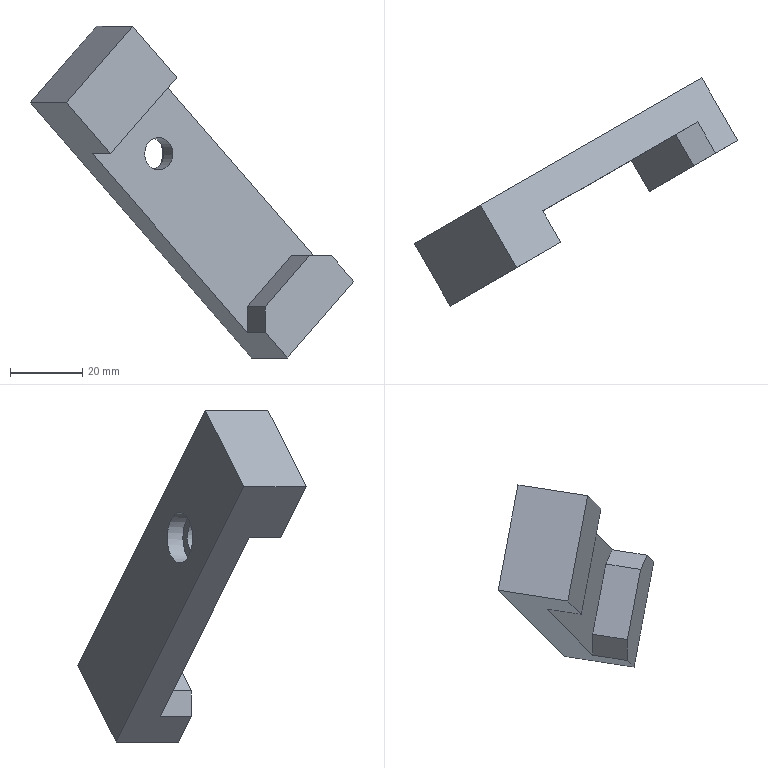Part | NX | features solid 2 | 1 solid | 15 faces | box 89.608 x 63.282 x 91.924 mm | volume 39162 mm3 | plane 13 | cylinder 2 | commonest cylinder face diameters 9 x1 14 x1
STEP:
#1=CARTESIAN_POINT('',(-1037.635,96.451,136.492));
#2=VERTEX_POINT('',#1);
#3=CARTESIAN_POINT('',(-1027.635,79.131,136.492));
#4=VERTEX_POINT('',#3);
#5=CARTESIAN_POINT('',(-1030.135,83.461,136.492));
#6=DIRECTION('',(0.5,-0.866,0.));
#7=VECTOR('',#6,1000.);
#8=LINE('',#5,#7);
#9=EDGE_CURVE('',#2,#4,#8,.T.);
#10=ORIENTED_EDGE('',*,*,#9,.T.);
#11=CARTESIAN_POINT('',(-1015.387,86.202,122.35));
#12=VERTEX_POINT('',#11);
#13=CARTESIAN_POINT('',(-1015.387,86.202,122.35));
#14=DIRECTION('',(-0.6124,-0.3536,0.7071));
#15=VECTOR('',#14,1000.);
#16=LINE('',#13,#15);
#17=EDGE_CURVE('',#4,#12,#16,.F.);
#18=ORIENTED_EDGE('',*,*,#17,.T.);
#19=CARTESIAN_POINT('',(-1020.387,94.862,122.35));
#20=VERTEX_POINT('',#19);
#21=CARTESIAN_POINT('',(-1017.887,90.532,122.35));
#22=DIRECTION('',(0.5,-0.866,0.));
#23=VECTOR('',#22,1000.);
#24=LINE('',#21,#23);
#25=EDGE_CURVE('',#20,#12,#24,.T.);
#26=ORIENTED_EDGE('',*,*,#25,.F.);
#27=CARTESIAN_POINT('',(-977.521,119.611,72.852));
#28=VERTEX_POINT('',#27);
#29=CARTESIAN_POINT('',(-1020.387,94.862,122.35));
#30=DIRECTION('',(-0.6124,-0.3536,0.7071));
#31=VECTOR('',#30,1000.);
#32=LINE('',#29,#31);
#33=EDGE_CURVE('',#20,#28,#32,.F.);
#34=ORIENTED_EDGE('',*,*,#33,.T.);
#35=CARTESIAN_POINT('',(-972.521,110.95,72.852));
#36=VERTEX_POINT('',#35);
#37=CARTESIAN_POINT('',(-975.021,115.28,72.852));
#38=DIRECTION('',(-0.5,0.866,0.));
#39=VECTOR('',#38,1000.);
#40=LINE('',#37,#39);
#41=EDGE_CURVE('',#36,#28,#40,.T.);
#42=ORIENTED_EDGE('',*,*,#41,.F.);
#43=CARTESIAN_POINT('',(-966.398,114.486,65.781));
#44=VERTEX_POINT('',#43);
#45=CARTESIAN_POINT('',(-1015.387,86.202,122.35));
#46=DIRECTION('',(0.6124,0.3536,-0.7071));
#47=VECTOR('',#46,1000.);
#48=LINE('',#45,#47);
#49=EDGE_CURVE('',#44,#36,#48,.F.);
#50=ORIENTED_EDGE('',*,*,#49,.F.);
#51=CARTESIAN_POINT('',(-976.398,131.806,65.781));
#52=VERTEX_POINT('',#51);
#53=CARTESIAN_POINT('',(-968.898,118.816,65.781));
#54=DIRECTION('',(0.5,-0.866,0.));
#55=VECTOR('',#54,1000.);
#56=LINE('',#53,#55);
#57=EDGE_CURVE('',#52,#44,#56,.T.);
#58=ORIENTED_EDGE('',*,*,#57,.F.);
#59=CARTESIAN_POINT('',(-1025.387,103.522,122.35));
#60=DIRECTION('',(-0.6124,-0.3536,0.7071));
#61=VECTOR('',#60,1000.);
#62=LINE('',#59,#61);
#63=EDGE_CURVE('',#52,#2,#62,.T.);
#64=ORIENTED_EDGE('',*,*,#63,.T.);
#65=EDGE_LOOP('',(#10,#18,#26,#34,#42,#50,#58,#64));
#66=FACE_BOUND('',#65,.T.);
#67=CARTESIAN_POINT('',(-1017.887,90.532,122.35));
#68=DIRECTION('',(0.6124,0.3536,0.7071));
#69=DIRECTION('',(0.5,-0.866,0.));
#70=AXIS2_PLACEMENT_3D('',#67,#68,#69);
#71=PLANE('',#70);
#72=ADVANCED_FACE('',(#66),#71,.T.);
#73=CARTESIAN_POINT('',(-1038.759,84.255,101.136));
#74=VERTEX_POINT('',#73);
#75=CARTESIAN_POINT('',(-1033.759,75.595,101.136));
#76=VERTEX_POINT('',#75);
#77=CARTESIAN_POINT('',(-1036.259,79.925,101.136));
#78=DIRECTION('',(-0.5,0.866,0.));
#79=VECTOR('',#78,1000.);
#80=LINE('',#77,#79);
#81=EDGE_CURVE('',#74,#76,#80,.F.);
#82=ORIENTED_EDGE('',*,*,#81,.T.);
#83=CARTESIAN_POINT('',(-1046.006,68.524,115.279));
#84=VERTEX_POINT('',#83);
#85=CARTESIAN_POINT('',(-1033.759,75.595,101.136));
#86=DIRECTION('',(-0.6124,-0.3536,0.7071));
#87=VECTOR('',#86,1000.);
#88=LINE('',#85,#87);
#89=EDGE_CURVE('',#76,#84,#88,.T.);
#90=ORIENTED_EDGE('',*,*,#89,.T.);
#91=CARTESIAN_POINT('',(-1056.006,85.844,115.279));
#92=VERTEX_POINT('',#91);
#93=CARTESIAN_POINT('',(-1048.506,72.854,115.279));
#94=DIRECTION('',(-0.5,0.866,0.));
#95=VECTOR('',#94,1000.);
#96=LINE('',#93,#95);
#97=EDGE_CURVE('',#92,#84,#96,.F.);
#98=ORIENTED_EDGE('',*,*,#97,.F.);
#99=CARTESIAN_POINT('',(-994.769,121.2,44.568));
#100=VERTEX_POINT('',#99);
#101=CARTESIAN_POINT('',(-1043.759,92.916,101.136));
#102=DIRECTION('',(0.6124,0.3536,-0.7071));
#103=VECTOR('',#102,1000.);
#104=LINE('',#101,#103);
#105=EDGE_CURVE('',#100,#92,#104,.F.);
#106=ORIENTED_EDGE('',*,*,#105,.F.);
#107=CARTESIAN_POINT('',(-984.769,103.879,44.568));
#108=VERTEX_POINT('',#107);
#109=CARTESIAN_POINT('',(-987.269,108.209,44.568));
#110=DIRECTION('',(-0.5,0.866,0.));
#111=VECTOR('',#110,1000.);
#112=LINE('',#109,#111);
#113=EDGE_CURVE('',#100,#108,#112,.F.);
#114=ORIENTED_EDGE('',*,*,#113,.T.);
#115=CARTESIAN_POINT('',(-990.893,100.344,51.639));
#116=VERTEX_POINT('',#115);
#117=CARTESIAN_POINT('',(-1033.759,75.595,101.136));
#118=DIRECTION('',(-0.6124,-0.3536,0.7071));
#119=VECTOR('',#118,1000.);
#120=LINE('',#117,#119);
#121=EDGE_CURVE('',#108,#116,#120,.T.);
#122=ORIENTED_EDGE('',*,*,#121,.T.);
#123=CARTESIAN_POINT('',(-995.893,109.004,51.639));
#124=VERTEX_POINT('',#123);
#125=CARTESIAN_POINT('',(-993.393,104.674,51.639));
#126=DIRECTION('',(-0.5,0.866,0.));
#127=VECTOR('',#126,1000.);
#128=LINE('',#125,#127);
#129=EDGE_CURVE('',#124,#116,#128,.F.);
#130=ORIENTED_EDGE('',*,*,#129,.F.);
#131=CARTESIAN_POINT('',(-1038.759,84.255,101.136));
#132=DIRECTION('',(0.6124,0.3536,-0.7071));
#133=VECTOR('',#132,1000.);
#134=LINE('',#131,#133);
#135=EDGE_CURVE('',#74,#124,#134,.T.);
#136=ORIENTED_EDGE('',*,*,#135,.F.);
#137=EDGE_LOOP('',(#82,#90,#98,#106,#114,#122,#130,#136));
#138=FACE_BOUND('',#137,.T.);
#139=CARTESIAN_POINT('',(-1036.259,79.925,101.136));
#140=DIRECTION('',(0.6124,0.3536,0.7071));
#141=DIRECTION('',(0.5,-0.866,0.));
#142=AXIS2_PLACEMENT_3D('',#139,#140,#141);
#143=PLANE('',#142);
#144=ADVANCED_FACE('',(#138),#143,.F.);
#145=ORIENTED_EDGE('',*,*,#97,.T.);
#146=CARTESIAN_POINT('',(-1052.13,64.988,108.208));
#147=DIRECTION('',(-0.6124,-0.3536,-0.7071));
#148=VECTOR('',#147,1000.);
#149=LINE('',#146,#148);
#150=EDGE_CURVE('',#84,#4,#149,.F.);
#151=ORIENTED_EDGE('',*,*,#150,.T.);
#152=ORIENTED_EDGE('',*,*,#9,.F.);
#153=CARTESIAN_POINT('',(-1062.13,82.309,108.208));
#154=DIRECTION('',(0.6124,0.3536,0.7071));
#155=VECTOR('',#154,1000.);
#156=LINE('',#153,#155);
#157=EDGE_CURVE('',#92,#2,#156,.T.);
#158=ORIENTED_EDGE('',*,*,#157,.F.);
#159=EDGE_LOOP('',(#145,#151,#152,#158));
#160=FACE_BOUND('',#159,.T.);
#161=CARTESIAN_POINT('',(-1054.63,69.319,108.208));
#162=DIRECTION('',(-0.6124,-0.3536,0.7071));
#163=DIRECTION('',(0.6124,0.3536,0.7071));
#164=AXIS2_PLACEMENT_3D('',#161,#162,#163);
#165=PLANE('',#164);
#166=ADVANCED_FACE('',(#160),#165,.T.);
#167=CARTESIAN_POINT('',(-1039.882,72.059,94.065));
#168=DIRECTION('',(-0.6124,-0.3536,-0.7071));
#169=VECTOR('',#168,1000.);
#170=LINE('',#167,#169);
#171=EDGE_CURVE('',#76,#12,#170,.F.);
#172=ORIENTED_EDGE('',*,*,#171,.F.);
#173=ORIENTED_EDGE('',*,*,#81,.F.);
#174=CARTESIAN_POINT('',(-1044.882,80.72,94.065));
#175=DIRECTION('',(-0.6124,-0.3536,-0.7071));
#176=VECTOR('',#175,1000.);
#177=LINE('',#174,#176);
#178=EDGE_CURVE('',#74,#20,#177,.F.);
#179=ORIENTED_EDGE('',*,*,#178,.T.);
#180=ORIENTED_EDGE('',*,*,#25,.T.);
#181=EDGE_LOOP('',(#172,#173,#179,#180));
#182=FACE_BOUND('',#181,.T.);
#183=CARTESIAN_POINT('',(-1042.382,76.39,94.065));
#184=DIRECTION('',(-0.6124,-0.3536,0.7071));
#185=DIRECTION('',(0.6124,0.3536,0.7071));
#186=AXIS2_PLACEMENT_3D('',#183,#184,#185);
#187=PLANE('',#186);
#188=ADVANCED_FACE('',(#182),#187,.F.);
#189=ORIENTED_EDGE('',*,*,#121,.F.);
#190=CARTESIAN_POINT('',(-990.893,100.344,37.497));
#191=DIRECTION('',(-0.6124,-0.3536,-0.7071));
#192=VECTOR('',#191,1000.);
#193=LINE('',#190,#192);
#194=EDGE_CURVE('',#108,#44,#193,.F.);
#195=ORIENTED_EDGE('',*,*,#194,.T.);
#196=ORIENTED_EDGE('',*,*,#49,.T.);
#197=CARTESIAN_POINT('',(-978.645,107.415,72.852));
#198=VERTEX_POINT('',#197);
#199=CARTESIAN_POINT('',(-978.645,107.415,72.852));
#200=DIRECTION('',(0.866,0.5,0.));
#201=VECTOR('',#200,1000.);
#202=LINE('',#199,#201);
#203=EDGE_CURVE('',#198,#36,#202,.T.);
#204=ORIENTED_EDGE('',*,*,#203,.F.);
#205=CARTESIAN_POINT('',(-990.893,100.344,58.71));
#206=VERTEX_POINT('',#205);
#207=CARTESIAN_POINT('',(-1000.078,95.04,48.103));
#208=DIRECTION('',(-0.6124,-0.3536,-0.7071));
#209=VECTOR('',#208,1000.);
#210=LINE('',#207,#209);
#211=EDGE_CURVE('',#206,#198,#210,.F.);
#212=ORIENTED_EDGE('',*,*,#211,.F.);
#213=CARTESIAN_POINT('',(-990.893,100.344,51.639));
#214=DIRECTION('',(0.,0.,-1.));
#215=VECTOR('',#214,1000.);
#216=LINE('',#213,#215);
#217=EDGE_CURVE('',#116,#206,#216,.F.);
#218=ORIENTED_EDGE('',*,*,#217,.F.);
#219=EDGE_LOOP('',(#189,#195,#196,#204,#212,#218));
#220=FACE_BOUND('',#219,.T.);
#221=CARTESIAN_POINT('',(-1039.882,72.059,94.065));
#222=DIRECTION('',(-0.5,0.866,0.));
#223=DIRECTION('',(0.6124,0.3536,0.7071));
#224=AXIS2_PLACEMENT_3D('',#221,#222,#223);
#225=PLANE('',#224);
#226=ADVANCED_FACE('',(#220),#225,.F.);
#227=CARTESIAN_POINT('',(-1025.916,103.217,108.11));
#228=VERTEX_POINT('',#227);
#229=CARTESIAN_POINT('',(-1025.387,103.522,101.136));
#230=DIRECTION('',(-0.5,0.866,0.));
#231=DIRECTION('',(-0.07548,-0.04358,0.9962));
#232=AXIS2_PLACEMENT_3D('',#229,#230,#231);
#233=CIRCLE('',#232,7.);
#234=EDGE_CURVE('',#228,#228,#233,.T.);
#235=ORIENTED_EDGE('',*,*,#234,.F.);
#236=EDGE_LOOP('',(#235));
#237=FACE_BOUND('',#236,.T.);
#238=ORIENTED_EDGE('',*,*,#105,.T.);
#239=ORIENTED_EDGE('',*,*,#157,.T.);
#240=ORIENTED_EDGE('',*,*,#63,.F.);
#241=CARTESIAN_POINT('',(-1000.893,117.664,37.497));
#242=DIRECTION('',(0.6124,0.3536,0.7071));
#243=VECTOR('',#242,1000.);
#244=LINE('',#241,#243);
#245=EDGE_CURVE('',#100,#52,#244,.T.);
#246=ORIENTED_EDGE('',*,*,#245,.F.);
#247=EDGE_LOOP('',(#238,#239,#240,#246));
#248=FACE_BOUND('',#247,.T.);
#249=CARTESIAN_POINT('',(-1049.882,89.38,94.065));
#250=DIRECTION('',(-0.5,0.866,0.));
#251=DIRECTION('',(0.6124,0.3536,0.7071));
#252=AXIS2_PLACEMENT_3D('',#249,#250,#251);
#253=PLANE('',#252);
#254=ADVANCED_FACE('',(#237,#248),#253,.T.);
#255=ORIENTED_EDGE('',*,*,#194,.F.);
#256=ORIENTED_EDGE('',*,*,#113,.F.);
#257=ORIENTED_EDGE('',*,*,#245,.T.);
#258=ORIENTED_EDGE('',*,*,#57,.T.);
#259=EDGE_LOOP('',(#255,#256,#257,#258));
#260=FACE_BOUND('',#259,.T.);
#261=CARTESIAN_POINT('',(-993.393,104.674,37.497));
#262=DIRECTION('',(-0.6124,-0.3536,0.7071));
#263=DIRECTION('',(0.6124,0.3536,0.7071));
#264=AXIS2_PLACEMENT_3D('',#261,#262,#263);
#265=PLANE('',#264);
#266=ADVANCED_FACE('',(#260),#265,.F.);
#267=CARTESIAN_POINT('',(-983.645,116.075,72.852));
#268=VERTEX_POINT('',#267);
#269=CARTESIAN_POINT('',(-1044.882,80.72,72.852));
#270=DIRECTION('',(-0.866,-0.5,0.));
#271=VECTOR('',#270,1000.);
#272=LINE('',#269,#271);
#273=EDGE_CURVE('',#28,#268,#272,.T.);
#274=ORIENTED_EDGE('',*,*,#273,.F.);
#275=ORIENTED_EDGE('',*,*,#33,.F.);
#276=ORIENTED_EDGE('',*,*,#178,.F.);
#277=ORIENTED_EDGE('',*,*,#135,.T.);
#278=CARTESIAN_POINT('',(-995.893,109.004,58.71));
#279=VERTEX_POINT('',#278);
#280=CARTESIAN_POINT('',(-995.893,109.004,94.065));
#281=DIRECTION('',(0.,0.,1.));
#282=VECTOR('',#281,1000.);
#283=LINE('',#280,#282);
#284=EDGE_CURVE('',#279,#124,#283,.F.);
#285=ORIENTED_EDGE('',*,*,#284,.F.);
#286=CARTESIAN_POINT('',(-1005.078,103.701,48.103));
#287=DIRECTION('',(-0.6124,-0.3536,-0.7071));
#288=VECTOR('',#287,1000.);
#289=LINE('',#286,#288);
#290=EDGE_CURVE('',#279,#268,#289,.F.);
#291=ORIENTED_EDGE('',*,*,#290,.T.);
#292=EDGE_LOOP('',(#274,#275,#276,#277,#285,#291));
#293=FACE_BOUND('',#292,.T.);
#294=CARTESIAN_POINT('',(-1024.27,92.62,101.529));
#295=VERTEX_POINT('',#294);
#296=CARTESIAN_POINT('',(-1020.387,94.862,101.136));
#297=DIRECTION('',(-0.5,0.866,0.));
#298=DIRECTION('',(-0.8627,-0.4981,0.08716));
#299=AXIS2_PLACEMENT_3D('',#296,#297,#298);
#300=CIRCLE('',#299,4.5);
#301=EDGE_CURVE('',#295,#295,#300,.T.);
#302=ORIENTED_EDGE('',*,*,#301,.T.);
#303=EDGE_LOOP('',(#302));
#304=FACE_BOUND('',#303,.T.);
#305=CARTESIAN_POINT('',(-1044.882,80.72,94.065));
#306=DIRECTION('',(-0.5,0.866,0.));
#307=DIRECTION('',(0.6124,0.3536,0.7071));
#308=AXIS2_PLACEMENT_3D('',#305,#306,#307);
#309=PLANE('',#308);
#310=ADVANCED_FACE('',(#293,#304),#309,.F.);
#311=ORIENTED_EDGE('',*,*,#211,.T.);
#312=CARTESIAN_POINT('',(-981.145,111.745,72.852));
#313=DIRECTION('',(0.5,-0.866,0.));
#314=VECTOR('',#313,1000.);
#315=LINE('',#312,#314);
#316=EDGE_CURVE('',#268,#198,#315,.T.);
#317=ORIENTED_EDGE('',*,*,#316,.F.);
#318=ORIENTED_EDGE('',*,*,#290,.F.);
#319=CARTESIAN_POINT('',(-993.393,104.674,58.71));
#320=DIRECTION('',(-0.5,0.866,0.));
#321=VECTOR('',#320,1000.);
#322=LINE('',#319,#321);
#323=EDGE_CURVE('',#206,#279,#322,.T.);
#324=ORIENTED_EDGE('',*,*,#323,.F.);
#325=EDGE_LOOP('',(#311,#317,#318,#324));
#326=FACE_BOUND('',#325,.T.);
#327=CARTESIAN_POINT('',(-1002.578,99.371,48.103));
#328=DIRECTION('',(-0.6124,-0.3536,0.7071));
#329=DIRECTION('',(0.6124,0.3536,0.7071));
#330=AXIS2_PLACEMENT_3D('',#327,#328,#329);
#331=PLANE('',#330);
#332=ADVANCED_FACE('',(#326),#331,.T.);
#333=ORIENTED_EDGE('',*,*,#284,.T.);
#334=ORIENTED_EDGE('',*,*,#129,.T.);
#335=ORIENTED_EDGE('',*,*,#217,.T.);
#336=ORIENTED_EDGE('',*,*,#323,.T.);
#337=EDGE_LOOP('',(#333,#334,#335,#336));
#338=FACE_BOUND('',#337,.T.);
#339=CARTESIAN_POINT('',(-993.393,104.674,51.639));
#340=DIRECTION('',(-0.866,-0.5,0.));
#341=DIRECTION('',(0.,0.,1.));
#342=AXIS2_PLACEMENT_3D('',#339,#340,#341);
#343=PLANE('',#342);
#344=ADVANCED_FACE('',(#338),#343,.T.);
#345=ORIENTED_EDGE('',*,*,#273,.T.);
#346=ORIENTED_EDGE('',*,*,#316,.T.);
#347=ORIENTED_EDGE('',*,*,#203,.T.);
#348=ORIENTED_EDGE('',*,*,#41,.T.);
#349=EDGE_LOOP('',(#345,#346,#347,#348));
#350=FACE_BOUND('',#349,.T.);
#351=CARTESIAN_POINT('',(-981.145,111.745,72.852));
#352=DIRECTION('',(0.,0.,-1.));
#353=DIRECTION('',(-0.866,-0.5,0.));
#354=AXIS2_PLACEMENT_3D('',#351,#352,#353);
#355=PLANE('',#354);
#356=ADVANCED_FACE('',(#350),#355,.F.);
#357=ORIENTED_EDGE('',*,*,#301,.F.);
#358=EDGE_LOOP('',(#357));
#359=FACE_BOUND('',#358,.T.);
#360=CARTESIAN_POINT('',(-1019.005,101.433,100.744));
#361=VERTEX_POINT('',#360);
#362=CARTESIAN_POINT('',(-1022.887,99.192,101.136));
#363=DIRECTION('',(0.5,-0.866,0.));
#364=DIRECTION('',(0.8627,0.4981,-0.08716));
#365=AXIS2_PLACEMENT_3D('',#362,#363,#364);
#366=CIRCLE('',#365,4.5);
#367=EDGE_CURVE('',#361,#361,#366,.F.);
#368=ORIENTED_EDGE('',*,*,#367,.T.);
#369=EDGE_LOOP('',(#368));
#370=FACE_BOUND('',#369,.T.);
#371=CARTESIAN_POINT('',(-1000.387,60.221,101.136));
#372=DIRECTION('',(0.5,-0.866,0.));
#373=DIRECTION('',(-0.07548,-0.04358,0.9962));
#374=AXIS2_PLACEMENT_3D('',#371,#372,#373);
#375=CYLINDRICAL_SURFACE('',#374,4.5);
#376=ADVANCED_FACE('',(#359,#370),#375,.F.);
#377=ORIENTED_EDGE('',*,*,#367,.F.);
#378=EDGE_LOOP('',(#377));
#379=FACE_BOUND('',#378,.T.);
#380=CARTESIAN_POINT('',(-1016.848,102.679,100.526));
#381=VERTEX_POINT('',#380);
#382=CARTESIAN_POINT('',(-1022.887,99.192,101.136));
#383=DIRECTION('',(0.5,-0.866,0.));
#384=DIRECTION('',(0.8627,0.4981,-0.08716));
#385=AXIS2_PLACEMENT_3D('',#382,#383,#384);
#386=CIRCLE('',#385,7.);
#387=EDGE_CURVE('',#381,#381,#386,.F.);
#388=ORIENTED_EDGE('',*,*,#387,.T.);
#389=EDGE_LOOP('',(#388));
#390=FACE_BOUND('',#389,.T.);
#391=CARTESIAN_POINT('',(-1022.887,99.192,101.136));
#392=DIRECTION('',(0.5,-0.866,0.));
#393=DIRECTION('',(-0.07548,-0.04358,0.9962));
#394=AXIS2_PLACEMENT_3D('',#391,#392,#393);
#395=PLANE('',#394);
#396=ADVANCED_FACE('',(#379,#390),#395,.F.);
#397=ORIENTED_EDGE('',*,*,#387,.F.);
#398=EDGE_LOOP('',(#397));
#399=FACE_BOUND('',#398,.T.);
#400=ORIENTED_EDGE('',*,*,#234,.T.);
#401=EDGE_LOOP('',(#400));
#402=FACE_BOUND('',#401,.T.);
#403=CARTESIAN_POINT('',(-1025.387,103.522,101.136));
#404=DIRECTION('',(0.5,-0.866,0.));
#405=DIRECTION('',(-0.07548,-0.04358,0.9962));
#406=AXIS2_PLACEMENT_3D('',#403,#404,#405);
#407=CYLINDRICAL_SURFACE('',#406,7.);
#408=ADVANCED_FACE('',(#399,#402),#407,.F.);
#409=ORIENTED_EDGE('',*,*,#150,.F.);
#410=ORIENTED_EDGE('',*,*,#89,.F.);
#411=ORIENTED_EDGE('',*,*,#171,.T.);
#412=ORIENTED_EDGE('',*,*,#17,.F.);
#413=EDGE_LOOP('',(#409,#410,#411,#412));
#414=FACE_BOUND('',#413,.T.);
#415=CARTESIAN_POINT('',(-1039.882,72.059,94.065));
#416=DIRECTION('',(-0.5,0.866,0.));
#417=DIRECTION('',(0.6124,0.3536,0.7071));
#418=AXIS2_PLACEMENT_3D('',#415,#416,#417);
#419=PLANE('',#418);
#420=ADVANCED_FACE('',(#414),#419,.F.);
#421=CLOSED_SHELL('',(#72,#144,#166,#188,#226,#254,#266,#310,#332,#344,#356,#376,#396,#408,#420));
#422=MANIFOLD_SOLID_BREP('',#421);
#423=(LENGTH_UNIT()NAMED_UNIT(*)SI_UNIT(.MILLI.,.METRE.));
#424=UNCERTAINTY_MEASURE_WITH_UNIT(LENGTH_MEASURE(0.00001),#423,'','');
#425=(NAMED_UNIT(*)PLANE_ANGLE_UNIT()SI_UNIT($,.RADIAN.));
#426=(NAMED_UNIT(*)SI_UNIT($,.STERADIAN.)SOLID_ANGLE_UNIT());
#427=(GEOMETRIC_REPRESENTATION_CONTEXT(3)GLOBAL_UNCERTAINTY_ASSIGNED_CONTEXT((#424))GLOBAL_UNIT_ASSIGNED_CONTEXT((#423,#425,#426))REPRESENTATION_CONTEXT('',''));
#428=ADVANCED_BREP_SHAPE_REPRESENTATION('',(#422),#427);